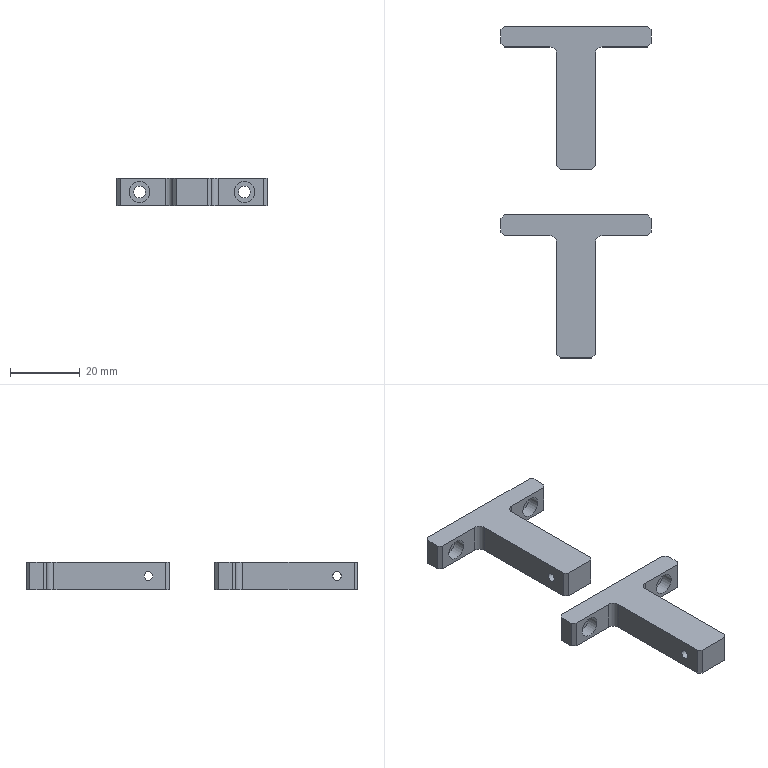NC program | NX | posted with a generic post | part box 43 x 95 x 8 mm
Whole program:
N10 G17 G21 G94 G90
(DRILLING_COPY_1_COPY_1 , TOOL : D6A45)
N12 T22 M6
N14 G54
N16 G17 G0 G90 X-15. Y0. B0. C0. S5000 M3
N18 G43 Z30. H22
N20 G94 G81 G98 Z-36. F250. R-32.
N22 X15.
N24 G80
N26 G0 X15. Y0. Z30.
N28 M5
(DRILLING_COPY_1_COPY_COPY_COPY_COPY_1_COPY_COPY_1_COPY_COPY_1_COPY , TOOL : 3.)
N30 T03 M6
N32 G54
N34 G17 G0 G90 X-15. Y0. B0. C0. S2000 M3
N36 G43 Z30. H3
N38 G94 G83 G98 Z-43.461 F150. Q2. R-32.
N40 X15.
N42 G80
N44 G0 X15. Y0. Z30.
N46 M5
(HOLE_MILLING_COPY_COPY_COPY , TOOL : D4)
N48 T15 M6
N50 G54
N52 G17 G0 G90 X-15. Y0. B0. C0. S7500 M3
N54 G43 Z30. H15
N56 Z-34.5
N58 G94 G3 X-14.5 Y-0.5 R0.5 F1000.
N60 X-14. Y0. R0.5
N62 X-14. Y0. Z-34.7 I-1. J0.
N64 X-14. Y0. Z-34.9 I-1. J0.
N66 X-14. Y0. Z-35.1 I-1. J0.
N68 X-14. Y0. Z-35.3 I-1. J0.
N70 X-14. Y0. Z-35.5 I-1. J0.
N72 X-14. Y0. Z-35.7 I-1. J0.
N74 X-14. Y0. Z-35.9 I-1. J0.
N76 X-14. Y0. Z-36.1 I-1. J0.
N78 X-14. Y0. Z-36.3 I-1. J0.
N80 X-14. Y0. Z-36.5 I-1. J0.
N82 X-14. Y0. Z-36.7 I-1. J0.
N84 X-14. Y0. Z-36.9 I-1. J0.
N86 X-14. Y0. Z-37.1 I-1. J0.
N88 X-14. Y0. Z-37.3 I-1. J0.
N90 X-14. Y0. Z-37.5 I-1. J0.
N92 X-14. Y0. Z-37.7 I-1. J0.
N94 X-14. Y0. Z-37.9 I-1. J0.
N96 X-14. Y0. Z-38.1 I-1. J0.
N98 X-14. Y0. Z-38.3 I-1. J0.
N100 X-16. Y0. Z-38.4 I-1. J0.
N102 X-15. Y-1. R1.
N104 X-16. Y0. R-1.
N106 X-15.5 Y-0.5 R0.5
N108 X-15. Y0. R0.5
N110 G0 Z30.
N112 X15.
N114 Z-34.5
N116 G3 X15.5 Y-0.5 R0.5
N118 X16. Y0. R0.5
N120 X16. Y0. Z-34.7 I-1. J0.
N122 X16. Y0. Z-34.9 I-1. J0.
N124 X16. Y0. Z-35.1 I-1. J0.
N126 X16. Y0. Z-35.3 I-1. J0.
N128 X16. Y0. Z-35.5 I-1. J0.
N130 X16. Y0. Z-35.7 I-1. J0.
N132 X16. Y0. Z-35.9 I-1. J0.
N134 X16. Y0. Z-36.1 I-1. J0.
N136 X16. Y0. Z-36.3 I-1. J0.
N138 X16. Y0. Z-36.5 I-1. J0.
N140 X16. Y0. Z-36.7 I-1. J0.
N142 X16. Y0. Z-36.9 I-1. J0.
N144 X16. Y0. Z-37.1 I-1. J0.
N146 X16. Y0. Z-37.3 I-1. J0.
N148 X16. Y0. Z-37.5 I-1. J0.
N150 X16. Y0. Z-37.7 I-1. J0.
N152 X16. Y0. Z-37.9 I-1. J0.
N154 X16. Y0. Z-38.1 I-1. J0.
N156 X16. Y0. Z-38.3 I-1. J0.
N158 X14. Y0. Z-38.4 I-1. J0.
N160 X15. Y-1. R1.
N162 X14. Y0. R-1.
N164 X14.5 Y-0.5 R0.5
N166 X15. Y0. R0.5
N168 G0 Z30.
N170 M5
N172 M2